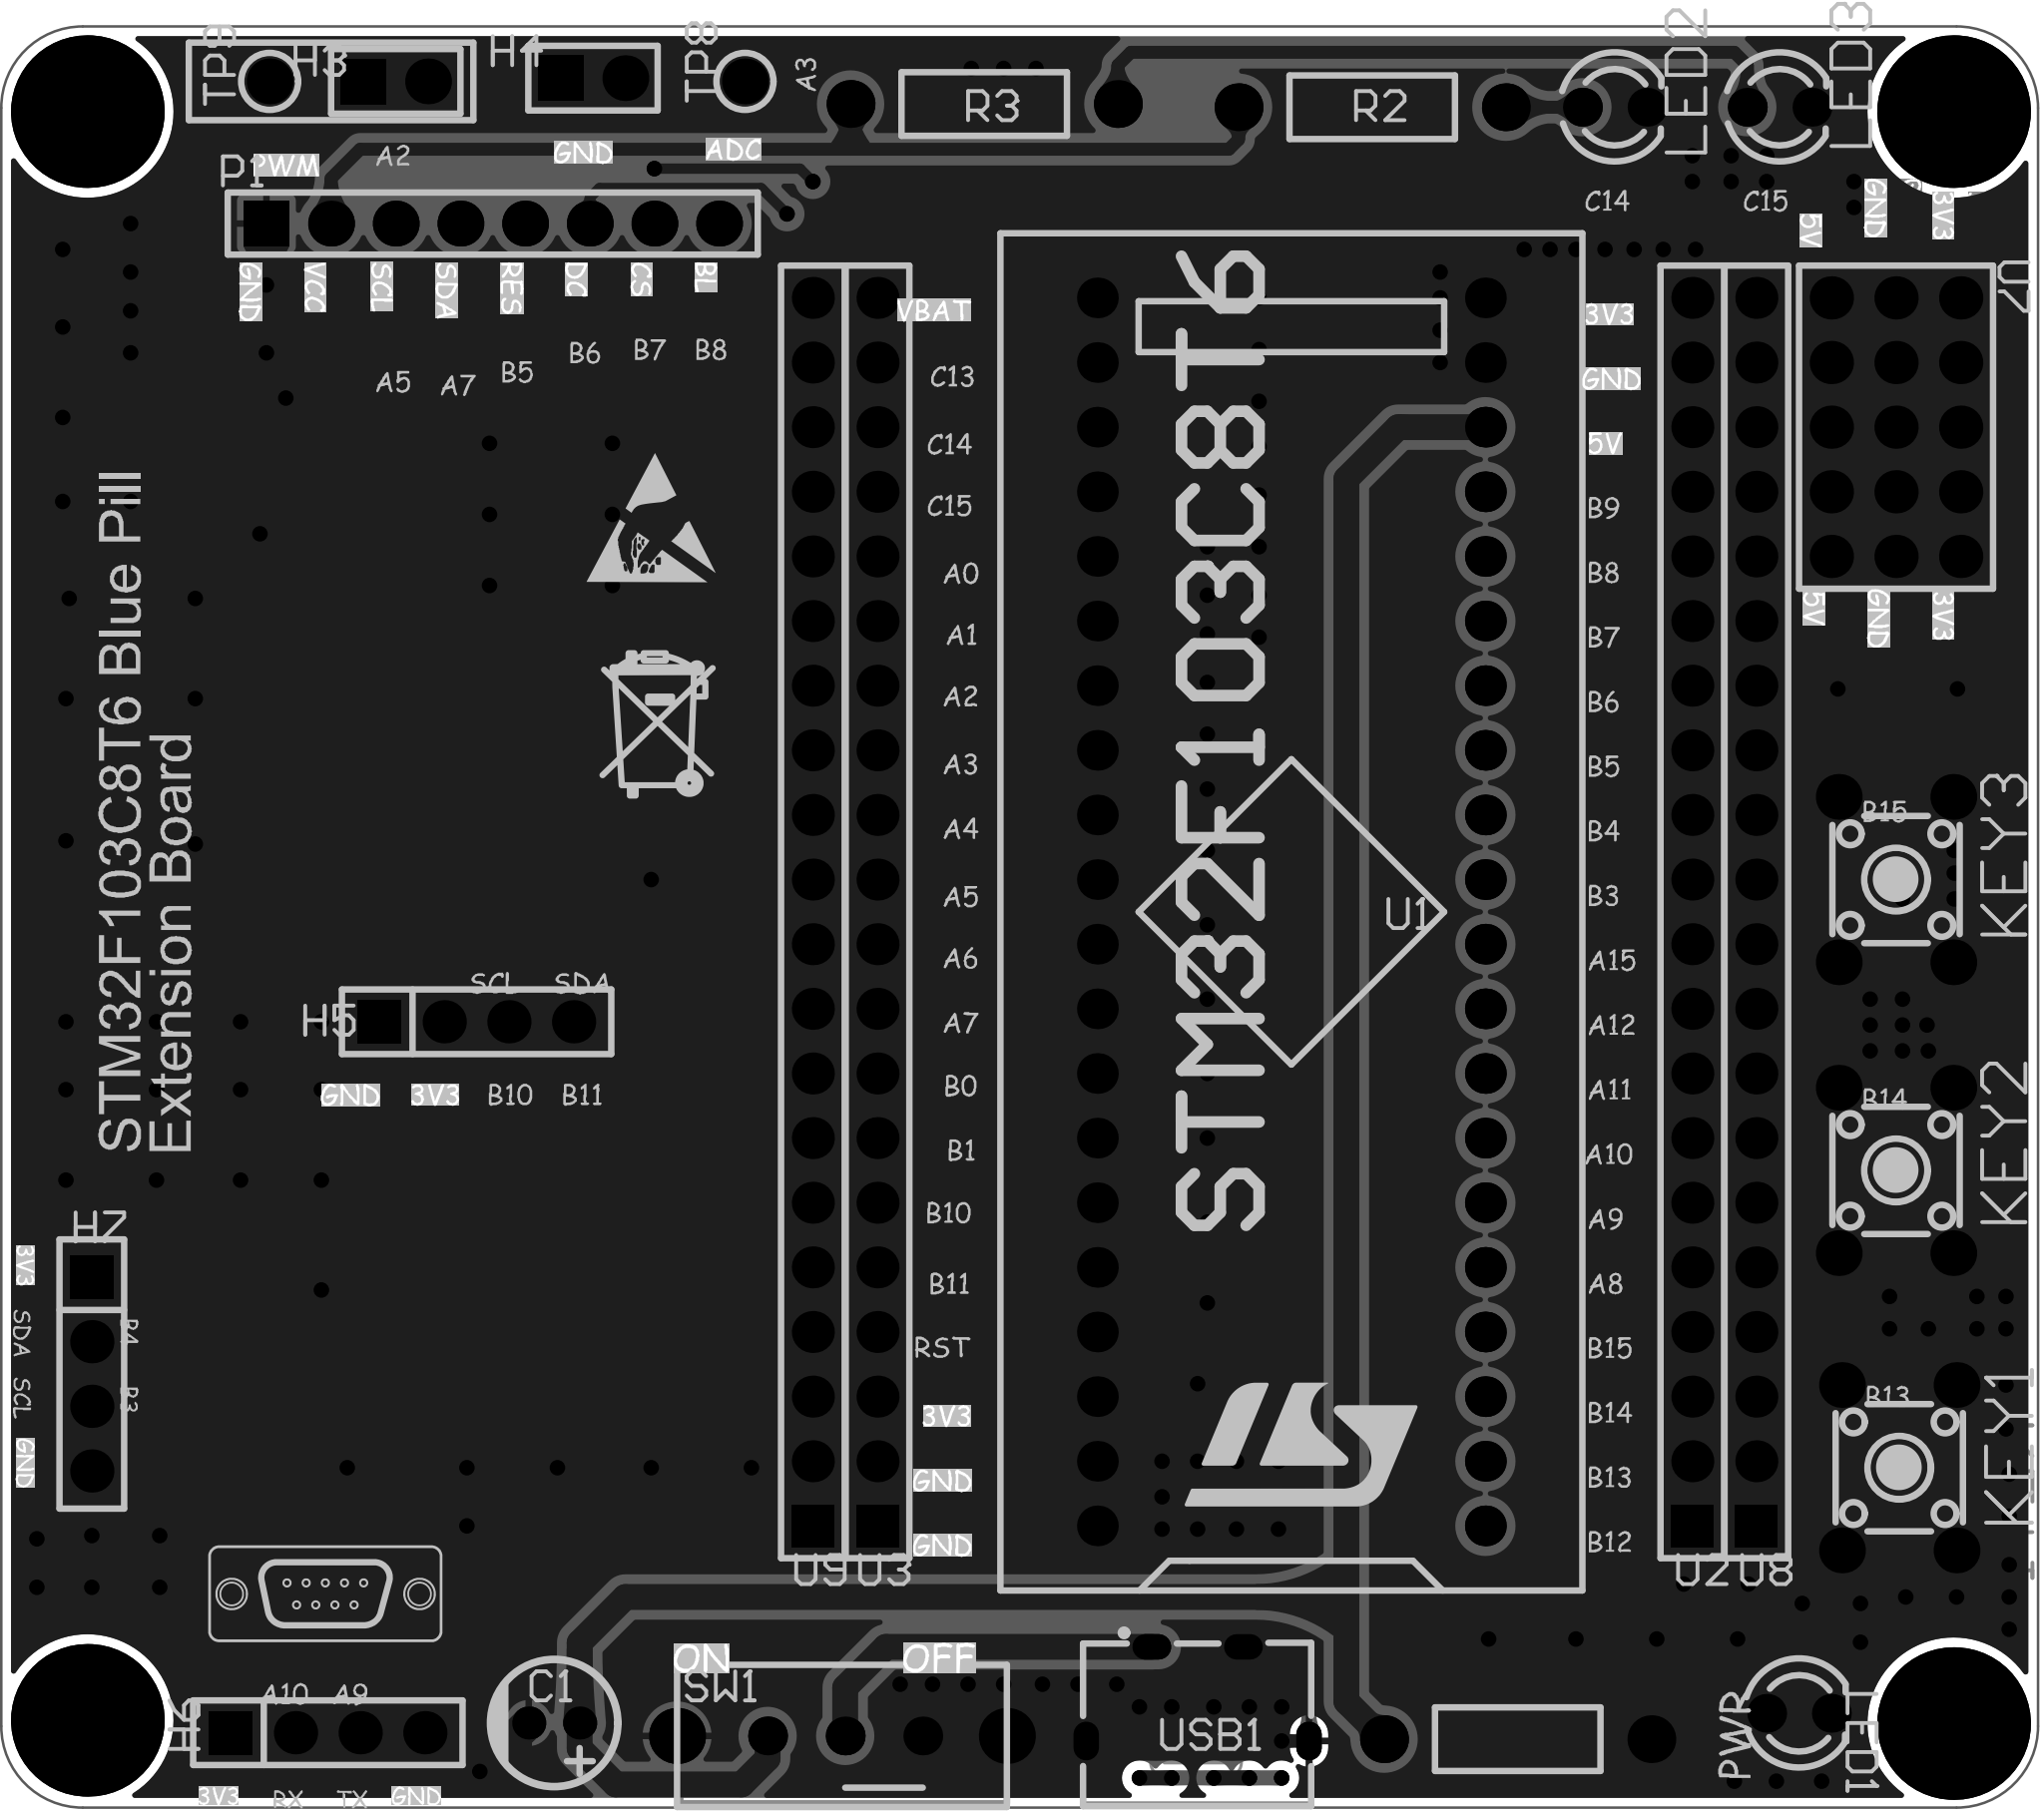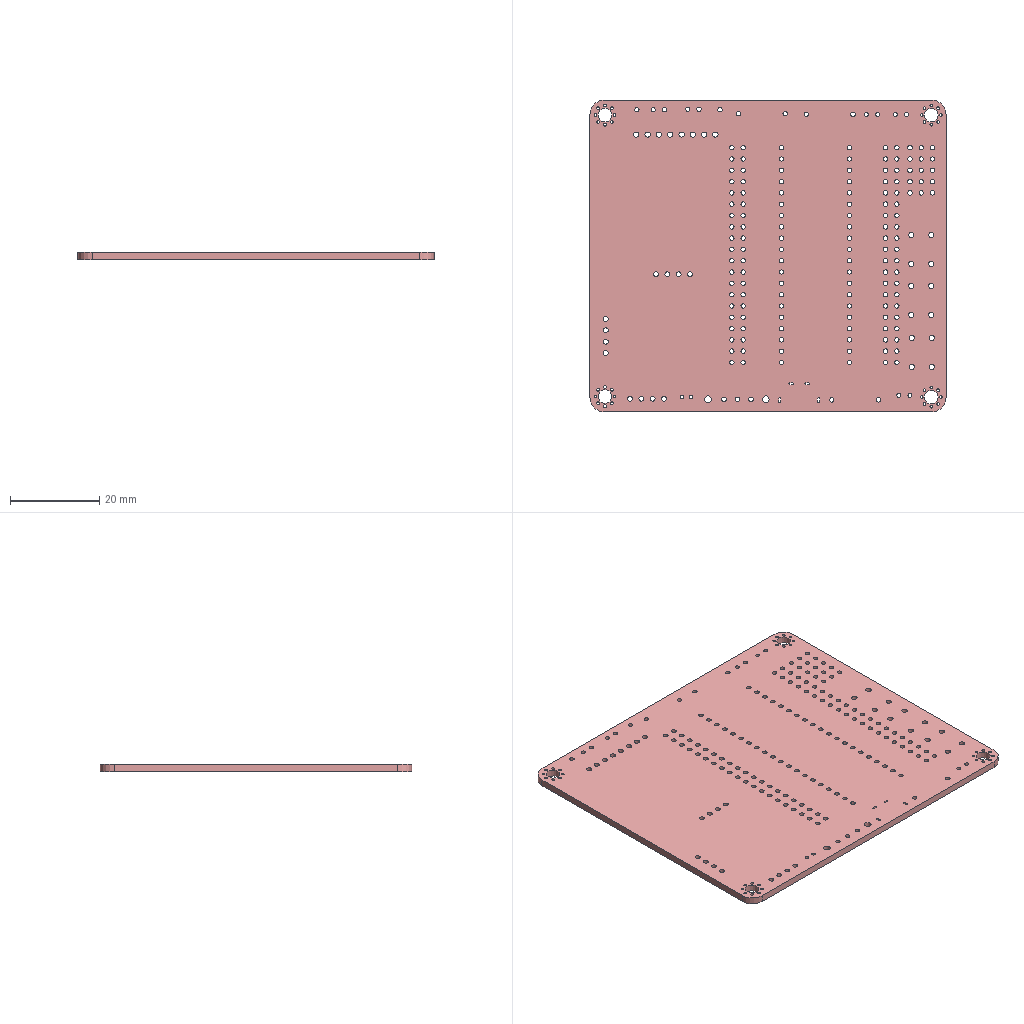Circuit board layout | Altium Designer | box 80 x 70 x 1.6 mm
Layer stack:
# Altium Designer layer stack of  (unit mm; dielectric type: 0 none, 1 core, 2 prepreg, 3 surface material)
index,name,kind,layer,copper_thickness_mm,dielectric_type,dielectric_thickness_mm,dielectric_material,dielectric_constant
0,Top Paste Mask Layer,other,,,,,,
1,Top Silkscreen Layer,other,,,,,,
2,Top Solder Mask Layer,dielectric,,,3,0.01,,3.3
3,Top Layer,copper,Top Layer,0.035,,,,
4,Dielectric1,dielectric,,,3,1.51,FR4,4.5
5,Bottom Layer,copper,Bottom Layer,0.035,,,,
6,Bottom Solder Mask Layer,dielectric,,,3,0.01,,3.3
7,Bottom Silkscreen Layer,other,,,,,,
8,Bottom Paste Mask Layer,other,,,,,,
# drill layer pairs: low layer,high layer
drill_pair,Top Layer,Bottom Layer
Part placement:
Designator,Comment,Layer,Footprint,Center-X(mm),Center-Y(mm),Rotation
H5,2.54-1*4P female,TopLayer,HDR-TH_4P-P2.54-V-F,95.758,112.522,0
R3,1kΩ,TopLayer,RES-TH_BD2.5-L6.5-P10.50-D0.6,115.697,148.59,180
U3,KH-2.54FH-1X20P-H8.5,TopLayer,HDR-TH_20P-P2.54-V-F-2,111.506,116.84,90
U1,LCKFB-DKX-STM32F103C8T6,TopLayer,CONN-TH_L53.3-W22.9_STM32F103C8T6-CARD,127.762,116.84,90
R2,1kΩ,TopLayer,RES-TH_BD2.5-L6.5-P10.50-D0.6,130.937,148.463,180
U2,KH-2.54FH-1X20P-H8.5,TopLayer,HDR-TH_20P-P2.54-V-F-2,143.51,116.84,90
LED2,,TopLayer,LED_TH-3mm,140.462,148.463,0
LED3,,TopLayer,LED_TH-3mm,146.939,148.463,0
KEY2,TC-6610-9-260G,TopLayer,SW-TH_4P-L5.0-W5.0-P4.50-LS6.5,151.511,106.68,90
KEY3,TC-6610-9-260G,TopLayer,SW-TH_4P-L5.0-W5.0-P4.50-LS6.5,151.511,118.11,90
KEY1,TC-6610-9-260G,TopLayer,SW-TH_4P-L5.0-W5.0-P4.50-LS6.5,151.638,94.996,90
H6,2.54-1*4P female,TopLayer,HDR-TH_4P-P2.54-V-F,89.916,84.582,0
H3,,TopLayer,HDR-TH_2P-P2.54-V-M-1,92.583,149.479,0
H4,,TopLayer,HDR-TH_2P-P2.54-V-M-1,100.33,149.606,0
TP9,TP-yellow test point,TopLayer,TESTPOINT-TH_BD3.2,87.63,149.479,0
TP8,TP-yellow test point,TopLayer,TESTPOINT-TH_BD3.2,106.299,149.479,0
K1,Flange pad,TopLayer,法兰焊盘-8孔-M3,80.47,85.068,0
K2,Flange pad,TopLayer,法兰焊盘-8孔-M3,153.772,84.941,0
K3,Flange pad,TopLayer,法兰焊盘-8孔-M3,80.47,148.291,0
K4,Flange pad,TopLayer,法兰焊盘-8孔-M3,153.772,148.291,0
C1,10uF,TopLayer,CAP-TH_BD5.0-P2.00-D0.8-FD,98.806,84.963,180
LED1,,TopLayer,LED_TH-3mm,147.701,85.344,0
R1,1kΩ,TopLayer,RES-TH_BD2.5-L6.5-P10.50-D0.6,136.652,84.328,180
SW1,SK-12E12-G5,TopLayer,SW-TH_SK-12E12-G5,110.109,84.455,270
USB1,KH-TYPE-C-2P,TopLayer,USB-SMD_KH-TYPE-C-2P,124.079,86.106,0
U7,HX PZ2.54-3x5P ZZ,TopLayer,HDR-TH_15P-P2.54-V-M-R3-C5-S7.5,151.511,135.89,270
P1,2.54-1*8P female RoHS,TopLayer,HDR-TH_8P-P2.54-V-F-1,96.393,143.891,0
U8,KH-2.54FH-1X20P-H8.5,TopLayer,HDR-TH_20P-P2.54-V-F-2,146.025,116.84,90
U9,KH-2.54FH-1X20P-H8.5,TopLayer,HDR-TH_20P-P2.54-V-F-2,108.966,116.84,90
H7,2.54-1*4P female,TopLayer,HDR-TH_4P-P2.54-V-F,80.645,98.679,270
Pad and via stacks:
# Altium Designer via and pad stacks of  (unit mm). Each distinct definition once, with the count of objects using it.
# via: kind,start_layer,end_layer,hole_mm,diameter_mm,mode(0 simple;1 top-mid-bottom;2 full stack),diameter_per_layer,count,example_net
# pad: kind,layer,hole_mm,hole_type(0 round;1 square;2 slot),plating,top_size,top_shape(1 round;2 rect;3 octagon;9 rounded rect),mid_size,bottom_size,mode,footprint,size_per_layer,count,example
pad,Multi-Layer,1.1,0,plated,1.7x1.7,2,1.7x1.7,1.7x1.7,0,HDR-TH_4P-P2.54-V-F,,3,H5.1
pad,Multi-Layer,1.1,0,plated,1.7x1.7,1,1.7x1.7,1.7x1.7,0,HDR-TH_4P-P2.54-V-F,,9,H5.2
pad,Multi-Layer,1,0,plated,1.88x1.88,1,1.88x1.88,1.88x1.88,0,RES-TH_BD2.5-L6.5-P10.50-D0.6,,6,R3.1
pad,Multi-Layer,1.02,0,plated,1.65x1.65,2,1.65x1.65,1.65x1.65,0,HDR-TH_20P-P2.54-V-F-2,,4,U3.1
pad,Multi-Layer,1.02,0,plated,1.65x1.65,1,1.65x1.65,1.65x1.65,0,HDR-TH_20P-P2.54-V-F-2,,76,U3.2
pad,Multi-Layer,1,0,plated,1.6x1.6,1,1.6x1.6,1.6x1.6,0,CONN-TH_L53.3-W22.9_STM32F103C8T6-CARD,,40,U1.1
pad,Multi-Layer,0.9144,0,plated,1.524x1.524,1,1.524x1.524,1.524x1.524,0,LED_TH-3mm,,6,LED2.1
pad,Multi-Layer,1.2,0,plated,1.8x1.8,1,1.8x1.8,1.8x1.8,0,SW-TH_4P-L5.0-W5.0-P4.50-LS6.5,,12,KEY2.1
pad,Multi-Layer,1,0,plated,1.8x1.8,1,1.8x1.8,1.8x1.8,0,HDR-TH_2P-P2.54-V-M-1,,2,H3.2
pad,Multi-Layer,1,0,plated,1.8x1.8,2,1.8x1.8,1.8x1.8,0,HDR-TH_2P-P2.54-V-M-1,,2,H3.1
pad,Multi-Layer,1,0,plated,1.8x1.8,1,1.8x1.8,1.8x1.8,0,TESTPOINT-TH_BD3.2,,2,TP9.1
pad,Multi-Layer,3.1,0,plated,6x6,1,6x6,6x6,0,\u00B7\u00A8\u00C0\u00BC\u00BA\u00B8\u00C5\u00CC-8\u00BF\u00D7-M3,,4,K1.1
pad,Multi-Layer,0.61,0,plated,1x1,1,1x1,1x1,0,\u00B7\u00A8\u00C0\u00BC\u00BA\u00B8\u00C5\u00CC-8\u00BF\u00D7-M3,,32,K1.1
pad,Multi-Layer,0.8,0,plated,1.3x1.3,1,1.3x1.3,1.3x1.3,0,CAP-TH_BD5.0-P2.00-D0.8-FD,,2,C1.1
pad,Multi-Layer,1,0,plated,1.524x1.524,1,1.524x1.524,1.524x1.524,0,SW-TH_SK-12E12-G5,,3,SW1.2
pad,Multi-Layer,1.5,0,plated,2.2x2.2,1,2.2x2.2,2.2x2.2,0,SW-TH_SK-12E12-G5,,2,SW1.4
pad,Multi-Layer,0.45,2,plated,1x1.524,1,1x1.524,1x1.524,0,USB-SMD_KH-TYPE-C-2P,,2,USB1.1
pad,Multi-Layer,0.5,2,plated,1x1.524,1,1x1.524,1x1.524,0,USB-SMD_KH-TYPE-C-2P,,2,USB1.3
pad,Multi-Layer,1,0,plated,1.7x1.7,1,1.7x1.7,1.7x1.7,0,HDR-TH_15P-P2.54-V-M-R3-C5-S7.5,,15,U7.1
pad,Multi-Layer,1.2,0,plated,1.8x1.8,2,1.8x1.8,1.8x1.8,0,HDR-TH_8P-P2.54-V-F-1,,1,P1.1
pad,Multi-Layer,1.2,0,plated,1.8x1.8,1,1.8x1.8,1.8x1.8,0,HDR-TH_8P-P2.54-V-F-1,,7,P1.2
via,Top Layer,Bottom Layer,0.3048,0.6096,0,,171,GND
Copper pours:
name,layer,net,type(0 solid;1 hatched;2 none)
Bottom Layer-GND,Bottom Layer,GND,0
Top Layer-GND,Top Layer,GND,0
Design rules, without the lines most boards share:
# Altium Designer design rules of  (exported by Altium Designer, unit mm)
# columns: name | kind | enabled | priority | scope1 | scope2 | descriptor | typed fields (field=value)
viaSize | 11 | enabled | 1 | All | All | Routing Via (MinHoleWidth=11.811mil) (MaxHoleWidth=248.032mil) (PreferredHoleWidth=12.008mil) (MinWidth=19.685mil) (MaxWidth=393.701mil) (PreferedWidth=24.016mil) (All) | via_min_hole=0.3 via_max_hole=6.3 via_preferred_diameter=0.61 via_preferred_hole=0.305
solderMaskExpansion | 13 | enabled | 2 | All | All | Solder Mask Expansion (Expansion =2.008mil) (All) | expansion=0.051